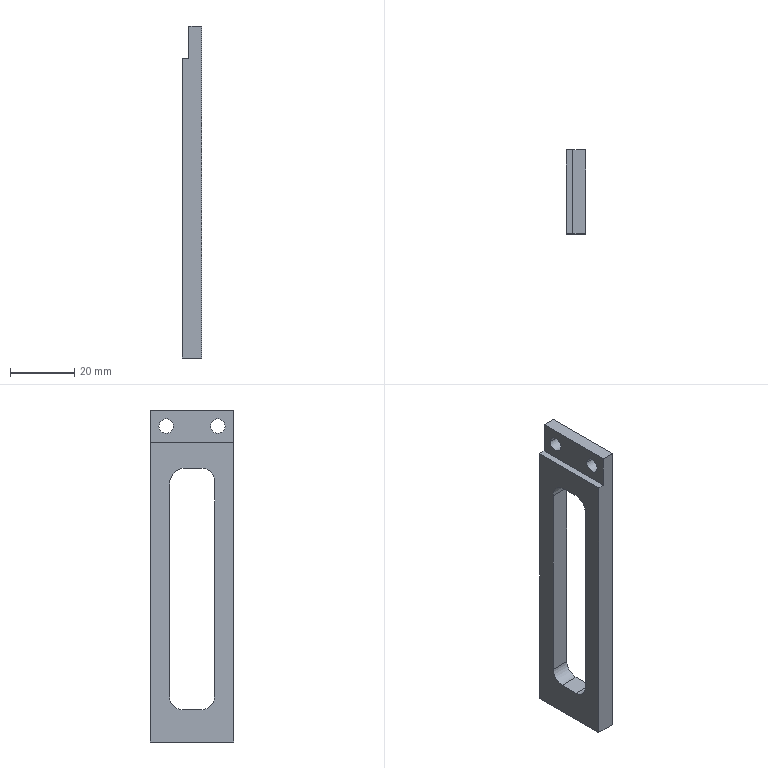Part | NX | 1 solid | 32 faces | box 6 x 26 x 103 mm | volume 9123 mm3 | plane 12 | cylinder 12 | cone 8 | commonest cylinder face diameters 2.5 x4 4.5 x4 8 x3 10 x1
STEP:
#1=CARTESIAN_POINT('',(594.,123.4,-250.82));
#2=VERTEX_POINT('',#1);
#3=CARTESIAN_POINT('',(592.,123.4,-250.82));
#4=VERTEX_POINT('',#3);
#5=CARTESIAN_POINT('',(594.,123.4,-250.82));
#6=DIRECTION('',(-1.,0.,0.));
#7=VECTOR('',#6,1000.);
#8=LINE('',#5,#7);
#9=EDGE_CURVE('',#2,#4,#8,.T.);
#10=ORIENTED_EDGE('',*,*,#9,.T.);
#11=CARTESIAN_POINT('',(592.,123.4,-343.82));
#12=VERTEX_POINT('',#11);
#13=CARTESIAN_POINT('',(592.,123.4,-246.201));
#14=DIRECTION('',(0.,0.,1.));
#15=VECTOR('',#14,1000.);
#16=LINE('',#13,#15);
#17=EDGE_CURVE('',#12,#4,#16,.T.);
#18=ORIENTED_EDGE('',*,*,#17,.F.);
#19=CARTESIAN_POINT('',(598.,123.4,-343.82));
#20=VERTEX_POINT('',#19);
#21=CARTESIAN_POINT('',(594.,123.4,-343.82));
#22=DIRECTION('',(1.,0.,0.));
#23=VECTOR('',#22,1000.);
#24=LINE('',#21,#23);
#25=EDGE_CURVE('',#12,#20,#24,.T.);
#26=ORIENTED_EDGE('',*,*,#25,.T.);
#27=CARTESIAN_POINT('',(598.,123.4,-240.82));
#28=VERTEX_POINT('',#27);
#29=CARTESIAN_POINT('',(598.,123.4,-246.201));
#30=DIRECTION('',(0.,0.,-1.));
#31=VECTOR('',#30,1000.);
#32=LINE('',#29,#31);
#33=EDGE_CURVE('',#28,#20,#32,.T.);
#34=ORIENTED_EDGE('',*,*,#33,.F.);
#35=CARTESIAN_POINT('',(594.,123.4,-240.82));
#36=VERTEX_POINT('',#35);
#37=CARTESIAN_POINT('',(594.,123.4,-240.82));
#38=DIRECTION('',(-1.,0.,0.));
#39=VECTOR('',#38,1000.);
#40=LINE('',#37,#39);
#41=EDGE_CURVE('',#28,#36,#40,.T.);
#42=ORIENTED_EDGE('',*,*,#41,.T.);
#43=CARTESIAN_POINT('',(594.,123.4,-246.201));
#44=DIRECTION('',(0.,0.,1.));
#45=VECTOR('',#44,1000.);
#46=LINE('',#43,#45);
#47=EDGE_CURVE('',#2,#36,#46,.T.);
#48=ORIENTED_EDGE('',*,*,#47,.F.);
#49=EDGE_LOOP('',(#10,#18,#26,#34,#42,#48));
#50=FACE_BOUND('',#49,.T.);
#51=CARTESIAN_POINT('',(594.,123.4,-250.82));
#52=DIRECTION('',(0.,-1.,0.));
#53=DIRECTION('',(0.,0.,-1.));
#54=AXIS2_PLACEMENT_3D('',#51,#52,#53);
#55=PLANE('',#54);
#56=ADVANCED_FACE('',(#50),#55,.T.);
#57=CARTESIAN_POINT('',(592.,149.4,-343.82));
#58=VERTEX_POINT('',#57);
#59=CARTESIAN_POINT('',(598.,149.4,-343.82));
#60=VERTEX_POINT('',#59);
#61=CARTESIAN_POINT('',(594.,149.4,-343.82));
#62=DIRECTION('',(1.,0.,0.));
#63=VECTOR('',#62,1000.);
#64=LINE('',#61,#63);
#65=EDGE_CURVE('',#58,#60,#64,.T.);
#66=ORIENTED_EDGE('',*,*,#65,.T.);
#67=CARTESIAN_POINT('',(598.,141.756,-343.82));
#68=DIRECTION('',(0.,1.,0.));
#69=VECTOR('',#68,1000.);
#70=LINE('',#67,#69);
#71=EDGE_CURVE('',#20,#60,#70,.T.);
#72=ORIENTED_EDGE('',*,*,#71,.F.);
#73=ORIENTED_EDGE('',*,*,#25,.F.);
#74=CARTESIAN_POINT('',(592.,141.756,-343.82));
#75=DIRECTION('',(0.,-1.,0.));
#76=VECTOR('',#75,1000.);
#77=LINE('',#74,#76);
#78=EDGE_CURVE('',#58,#12,#77,.T.);
#79=ORIENTED_EDGE('',*,*,#78,.F.);
#80=EDGE_LOOP('',(#66,#72,#73,#79));
#81=FACE_BOUND('',#80,.T.);
#82=CARTESIAN_POINT('',(596.6,126.9,-343.82));
#83=VERTEX_POINT('',#82);
#84=CARTESIAN_POINT('',(593.2,126.9,-343.82));
#85=VERTEX_POINT('',#84);
#86=CARTESIAN_POINT('',(594.9,126.9,-343.82));
#87=DIRECTION('',(0.,0.,-1.));
#88=DIRECTION('',(0.,-1.,0.));
#89=AXIS2_PLACEMENT_3D('',#86,#87,#88);
#90=CIRCLE('',#89,1.7);
#91=EDGE_CURVE('',#83,#85,#90,.T.);
#92=ORIENTED_EDGE('',*,*,#91,.F.);
#93=CARTESIAN_POINT('',(594.9,126.9,-343.82));
#94=DIRECTION('',(0.,0.,-1.));
#95=DIRECTION('',(0.,-1.,0.));
#96=AXIS2_PLACEMENT_3D('',#93,#94,#95);
#97=CIRCLE('',#96,1.7);
#98=EDGE_CURVE('',#85,#83,#97,.T.);
#99=ORIENTED_EDGE('',*,*,#98,.F.);
#100=EDGE_LOOP('',(#92,#99));
#101=FACE_BOUND('',#100,.T.);
#102=CARTESIAN_POINT('',(596.6,145.9,-343.82));
#103=VERTEX_POINT('',#102);
#104=CARTESIAN_POINT('',(593.2,145.9,-343.82));
#105=VERTEX_POINT('',#104);
#106=CARTESIAN_POINT('',(594.9,145.9,-343.82));
#107=DIRECTION('',(0.,0.,-1.));
#108=DIRECTION('',(0.,-1.,0.));
#109=AXIS2_PLACEMENT_3D('',#106,#107,#108);
#110=CIRCLE('',#109,1.7);
#111=EDGE_CURVE('',#103,#105,#110,.T.);
#112=ORIENTED_EDGE('',*,*,#111,.F.);
#113=CARTESIAN_POINT('',(594.9,145.9,-343.82));
#114=DIRECTION('',(0.,0.,-1.));
#115=DIRECTION('',(0.,-1.,0.));
#116=AXIS2_PLACEMENT_3D('',#113,#114,#115);
#117=CIRCLE('',#116,1.7);
#118=EDGE_CURVE('',#105,#103,#117,.T.);
#119=ORIENTED_EDGE('',*,*,#118,.F.);
#120=EDGE_LOOP('',(#112,#119));
#121=FACE_BOUND('',#120,.T.);
#122=CARTESIAN_POINT('',(594.,146.4,-343.82));
#123=DIRECTION('',(0.,0.,-1.));
#124=DIRECTION('',(0.,-1.,0.));
#125=AXIS2_PLACEMENT_3D('',#122,#123,#124);
#126=PLANE('',#125);
#127=ADVANCED_FACE('',(#81,#101,#121),#126,.T.);
#128=CARTESIAN_POINT('',(594.,149.4,-240.82));
#129=VERTEX_POINT('',#128);
#130=CARTESIAN_POINT('',(594.,149.4,-250.82));
#131=VERTEX_POINT('',#130);
#132=CARTESIAN_POINT('',(594.,149.4,-246.201));
#133=DIRECTION('',(0.,0.,-1.));
#134=VECTOR('',#133,1000.);
#135=LINE('',#132,#134);
#136=EDGE_CURVE('',#129,#131,#135,.T.);
#137=ORIENTED_EDGE('',*,*,#136,.F.);
#138=CARTESIAN_POINT('',(598.,149.4,-240.82));
#139=VERTEX_POINT('',#138);
#140=CARTESIAN_POINT('',(594.,149.4,-240.82));
#141=DIRECTION('',(1.,0.,0.));
#142=VECTOR('',#141,1000.);
#143=LINE('',#140,#142);
#144=EDGE_CURVE('',#129,#139,#143,.T.);
#145=ORIENTED_EDGE('',*,*,#144,.T.);
#146=CARTESIAN_POINT('',(598.,149.4,-246.201));
#147=DIRECTION('',(0.,0.,1.));
#148=VECTOR('',#147,1000.);
#149=LINE('',#146,#148);
#150=EDGE_CURVE('',#60,#139,#149,.T.);
#151=ORIENTED_EDGE('',*,*,#150,.F.);
#152=ORIENTED_EDGE('',*,*,#65,.F.);
#153=CARTESIAN_POINT('',(592.,149.4,-250.82));
#154=VERTEX_POINT('',#153);
#155=CARTESIAN_POINT('',(592.,149.4,-246.201));
#156=DIRECTION('',(0.,0.,-1.));
#157=VECTOR('',#156,1000.);
#158=LINE('',#155,#157);
#159=EDGE_CURVE('',#154,#58,#158,.T.);
#160=ORIENTED_EDGE('',*,*,#159,.F.);
#161=CARTESIAN_POINT('',(594.,149.4,-250.82));
#162=DIRECTION('',(1.,0.,0.));
#163=VECTOR('',#162,1000.);
#164=LINE('',#161,#163);
#165=EDGE_CURVE('',#154,#131,#164,.T.);
#166=ORIENTED_EDGE('',*,*,#165,.T.);
#167=EDGE_LOOP('',(#137,#145,#151,#152,#160,#166));
#168=FACE_BOUND('',#167,.T.);
#169=CARTESIAN_POINT('',(594.,149.4,-240.82));
#170=DIRECTION('',(0.,1.,0.));
#171=DIRECTION('',(1.,0.,0.));
#172=AXIS2_PLACEMENT_3D('',#169,#170,#171);
#173=PLANE('',#172);
#174=ADVANCED_FACE('',(#168),#173,.T.);
#175=CARTESIAN_POINT('',(594.,141.756,-240.82));
#176=DIRECTION('',(0.,1.,0.));
#177=VECTOR('',#176,1000.);
#178=LINE('',#175,#177);
#179=EDGE_CURVE('',#36,#129,#178,.T.);
#180=ORIENTED_EDGE('',*,*,#179,.F.);
#181=ORIENTED_EDGE('',*,*,#41,.F.);
#182=CARTESIAN_POINT('',(598.,141.756,-240.82));
#183=DIRECTION('',(0.,-1.,0.));
#184=VECTOR('',#183,1000.);
#185=LINE('',#182,#184);
#186=EDGE_CURVE('',#139,#28,#185,.T.);
#187=ORIENTED_EDGE('',*,*,#186,.F.);
#188=ORIENTED_EDGE('',*,*,#144,.F.);
#189=EDGE_LOOP('',(#180,#181,#187,#188));
#190=FACE_BOUND('',#189,.T.);
#191=CARTESIAN_POINT('',(594.,126.4,-240.82));
#192=DIRECTION('',(0.,0.,1.));
#193=DIRECTION('',(1.,0.,0.));
#194=AXIS2_PLACEMENT_3D('',#191,#192,#193);
#195=PLANE('',#194);
#196=ADVANCED_FACE('',(#190),#195,.T.);
#197=CARTESIAN_POINT('',(592.,141.756,-250.82));
#198=DIRECTION('',(0.,1.,0.));
#199=VECTOR('',#198,1000.);
#200=LINE('',#197,#199);
#201=EDGE_CURVE('',#4,#154,#200,.T.);
#202=ORIENTED_EDGE('',*,*,#201,.T.);
#203=ORIENTED_EDGE('',*,*,#159,.T.);
#204=ORIENTED_EDGE('',*,*,#78,.T.);
#205=ORIENTED_EDGE('',*,*,#17,.T.);
#206=EDGE_LOOP('',(#202,#203,#204,#205));
#207=FACE_BOUND('',#206,.T.);
#208=CARTESIAN_POINT('',(592.,129.4,-329.82));
#209=VERTEX_POINT('',#208);
#210=CARTESIAN_POINT('',(592.,129.4,-262.82));
#211=VERTEX_POINT('',#210);
#212=CARTESIAN_POINT('',(592.,129.4,-246.201));
#213=DIRECTION('',(0.,0.,1.));
#214=VECTOR('',#213,1000.);
#215=LINE('',#212,#214);
#216=EDGE_CURVE('',#209,#211,#215,.T.);
#217=ORIENTED_EDGE('',*,*,#216,.F.);
#218=CARTESIAN_POINT('',(592.,133.4,-333.82));
#219=VERTEX_POINT('',#218);
#220=CARTESIAN_POINT('',(592.,133.4,-329.82));
#221=DIRECTION('',(-1.,0.,0.));
#222=DIRECTION('',(0.,-1.,0.));
#223=AXIS2_PLACEMENT_3D('',#220,#221,#222);
#224=CIRCLE('',#223,4.);
#225=EDGE_CURVE('',#219,#209,#224,.T.);
#226=ORIENTED_EDGE('',*,*,#225,.F.);
#227=CARTESIAN_POINT('',(592.,139.4,-333.82));
#228=VERTEX_POINT('',#227);
#229=CARTESIAN_POINT('',(592.,141.756,-333.82));
#230=DIRECTION('',(0.,-1.,0.));
#231=VECTOR('',#230,1000.);
#232=LINE('',#229,#231);
#233=EDGE_CURVE('',#228,#219,#232,.T.);
#234=ORIENTED_EDGE('',*,*,#233,.F.);
#235=CARTESIAN_POINT('',(592.,143.4,-329.82));
#236=VERTEX_POINT('',#235);
#237=CARTESIAN_POINT('',(592.,139.4,-329.82));
#238=DIRECTION('',(1.,0.,0.));
#239=DIRECTION('',(0.,1.,0.));
#240=AXIS2_PLACEMENT_3D('',#237,#238,#239);
#241=CIRCLE('',#240,4.);
#242=EDGE_CURVE('',#228,#236,#241,.T.);
#243=ORIENTED_EDGE('',*,*,#242,.T.);
#244=CARTESIAN_POINT('',(592.,143.4,-263.82));
#245=VERTEX_POINT('',#244);
#246=CARTESIAN_POINT('',(592.,143.4,-246.201));
#247=DIRECTION('',(0.,0.,-1.));
#248=VECTOR('',#247,1000.);
#249=LINE('',#246,#248);
#250=EDGE_CURVE('',#245,#236,#249,.T.);
#251=ORIENTED_EDGE('',*,*,#250,.F.);
#252=CARTESIAN_POINT('',(592.,138.4,-258.82));
#253=VERTEX_POINT('',#252);
#254=CARTESIAN_POINT('',(592.,138.4,-263.82));
#255=DIRECTION('',(1.,0.,0.));
#256=DIRECTION('',(0.,1.,0.));
#257=AXIS2_PLACEMENT_3D('',#254,#255,#256);
#258=CIRCLE('',#257,5.);
#259=EDGE_CURVE('',#245,#253,#258,.T.);
#260=ORIENTED_EDGE('',*,*,#259,.T.);
#261=CARTESIAN_POINT('',(592.,133.4,-258.82));
#262=VERTEX_POINT('',#261);
#263=CARTESIAN_POINT('',(592.,141.756,-258.82));
#264=DIRECTION('',(0.,1.,0.));
#265=VECTOR('',#264,1000.);
#266=LINE('',#263,#265);
#267=EDGE_CURVE('',#262,#253,#266,.T.);
#268=ORIENTED_EDGE('',*,*,#267,.F.);
#269=CARTESIAN_POINT('',(592.,133.4,-262.82));
#270=DIRECTION('',(1.,0.,0.));
#271=DIRECTION('',(0.,1.,0.));
#272=AXIS2_PLACEMENT_3D('',#269,#270,#271);
#273=CIRCLE('',#272,4.);
#274=EDGE_CURVE('',#262,#211,#273,.T.);
#275=ORIENTED_EDGE('',*,*,#274,.T.);
#276=EDGE_LOOP('',(#217,#226,#234,#243,#251,#260,#268,#275));
#277=FACE_BOUND('',#276,.T.);
#278=CARTESIAN_POINT('',(592.,137.557,-267.86));
#279=DIRECTION('',(-1.,0.,0.));
#280=DIRECTION('',(0.,0.,1.));
#281=AXIS2_PLACEMENT_3D('',#278,#279,#280);
#282=PLANE('',#281);
#283=ADVANCED_FACE('',(#207,#277),#282,.T.);
#284=CARTESIAN_POINT('',(598.,133.4,-258.82));
#285=VERTEX_POINT('',#284);
#286=CARTESIAN_POINT('',(594.,133.4,-258.82));
#287=DIRECTION('',(1.,0.,0.));
#288=VECTOR('',#287,1000.);
#289=LINE('',#286,#288);
#290=EDGE_CURVE('',#262,#285,#289,.T.);
#291=ORIENTED_EDGE('',*,*,#290,.F.);
#292=ORIENTED_EDGE('',*,*,#267,.T.);
#293=CARTESIAN_POINT('',(598.,138.4,-258.82));
#294=VERTEX_POINT('',#293);
#295=CARTESIAN_POINT('',(594.,138.4,-258.82));
#296=DIRECTION('',(1.,0.,0.));
#297=VECTOR('',#296,1000.);
#298=LINE('',#295,#297);
#299=EDGE_CURVE('',#253,#294,#298,.T.);
#300=ORIENTED_EDGE('',*,*,#299,.T.);
#301=CARTESIAN_POINT('',(598.,141.756,-258.82));
#302=DIRECTION('',(0.,-1.,0.));
#303=VECTOR('',#302,1000.);
#304=LINE('',#301,#303);
#305=EDGE_CURVE('',#294,#285,#304,.T.);
#306=ORIENTED_EDGE('',*,*,#305,.T.);
#307=EDGE_LOOP('',(#291,#292,#300,#306));
#308=FACE_BOUND('',#307,.T.);
#309=CARTESIAN_POINT('',(591.4,129.4,-258.82));
#310=DIRECTION('',(0.,0.,1.));
#311=DIRECTION('',(1.,0.,0.));
#312=AXIS2_PLACEMENT_3D('',#309,#310,#311);
#313=PLANE('',#312);
#314=ADVANCED_FACE('',(#308),#313,.F.);
#315=CARTESIAN_POINT('',(598.,129.4,-329.82));
#316=VERTEX_POINT('',#315);
#317=CARTESIAN_POINT('',(594.,129.4,-329.82));
#318=DIRECTION('',(-1.,0.,0.));
#319=VECTOR('',#318,1000.);
#320=LINE('',#317,#319);
#321=EDGE_CURVE('',#316,#209,#320,.T.);
#322=ORIENTED_EDGE('',*,*,#321,.T.);
#323=ORIENTED_EDGE('',*,*,#216,.T.);
#324=CARTESIAN_POINT('',(598.,129.4,-262.82));
#325=VERTEX_POINT('',#324);
#326=CARTESIAN_POINT('',(594.,129.4,-262.82));
#327=DIRECTION('',(1.,0.,0.));
#328=VECTOR('',#327,1000.);
#329=LINE('',#326,#328);
#330=EDGE_CURVE('',#211,#325,#329,.T.);
#331=ORIENTED_EDGE('',*,*,#330,.T.);
#332=CARTESIAN_POINT('',(598.,129.4,-246.201));
#333=DIRECTION('',(0.,0.,-1.));
#334=VECTOR('',#333,1000.);
#335=LINE('',#332,#334);
#336=EDGE_CURVE('',#325,#316,#335,.T.);
#337=ORIENTED_EDGE('',*,*,#336,.T.);
#338=EDGE_LOOP('',(#322,#323,#331,#337));
#339=FACE_BOUND('',#338,.T.);
#340=CARTESIAN_POINT('',(591.4,129.4,-331.82));
#341=DIRECTION('',(0.,-1.,0.));
#342=DIRECTION('',(0.,0.,-1.));
#343=AXIS2_PLACEMENT_3D('',#340,#341,#342);
#344=PLANE('',#343);
#345=ADVANCED_FACE('',(#339),#344,.F.);
#346=CARTESIAN_POINT('',(598.,143.4,-329.82));
#347=VERTEX_POINT('',#346);
#348=CARTESIAN_POINT('',(594.,143.4,-329.82));
#349=DIRECTION('',(1.,0.,0.));
#350=VECTOR('',#349,1000.);
#351=LINE('',#348,#350);
#352=EDGE_CURVE('',#236,#347,#351,.T.);
#353=ORIENTED_EDGE('',*,*,#352,.T.);
#354=CARTESIAN_POINT('',(598.,143.4,-263.82));
#355=VERTEX_POINT('',#354);
#356=CARTESIAN_POINT('',(598.,143.4,-246.201));
#357=DIRECTION('',(0.,0.,1.));
#358=VECTOR('',#357,1000.);
#359=LINE('',#356,#358);
#360=EDGE_CURVE('',#347,#355,#359,.T.);
#361=ORIENTED_EDGE('',*,*,#360,.T.);
#362=CARTESIAN_POINT('',(594.,143.4,-263.82));
#363=DIRECTION('',(1.,0.,0.));
#364=VECTOR('',#363,1000.);
#365=LINE('',#362,#364);
#366=EDGE_CURVE('',#245,#355,#365,.T.);
#367=ORIENTED_EDGE('',*,*,#366,.F.);
#368=ORIENTED_EDGE('',*,*,#250,.T.);
#369=EDGE_LOOP('',(#353,#361,#367,#368));
#370=FACE_BOUND('',#369,.T.);
#371=CARTESIAN_POINT('',(591.4,143.4,-258.82));
#372=DIRECTION('',(0.,1.,0.));
#373=DIRECTION('',(1.,0.,0.));
#374=AXIS2_PLACEMENT_3D('',#371,#372,#373);
#375=PLANE('',#374);
#376=ADVANCED_FACE('',(#370),#375,.F.);
#377=CARTESIAN_POINT('',(598.,133.4,-333.82));
#378=VERTEX_POINT('',#377);
#379=CARTESIAN_POINT('',(598.,139.4,-333.82));
#380=VERTEX_POINT('',#379);
#381=CARTESIAN_POINT('',(598.,141.756,-333.82));
#382=DIRECTION('',(0.,1.,0.));
#383=VECTOR('',#382,1000.);
#384=LINE('',#381,#383);
#385=EDGE_CURVE('',#378,#380,#384,.T.);
#386=ORIENTED_EDGE('',*,*,#385,.T.);
#387=CARTESIAN_POINT('',(594.,139.4,-333.82));
#388=DIRECTION('',(1.,0.,0.));
#389=VECTOR('',#388,1000.);
#390=LINE('',#387,#389);
#391=EDGE_CURVE('',#228,#380,#390,.T.);
#392=ORIENTED_EDGE('',*,*,#391,.F.);
#393=ORIENTED_EDGE('',*,*,#233,.T.);
#394=CARTESIAN_POINT('',(594.,133.4,-333.82));
#395=DIRECTION('',(-1.,0.,0.));
#396=VECTOR('',#395,1000.);
#397=LINE('',#394,#396);
#398=EDGE_CURVE('',#378,#219,#397,.T.);
#399=ORIENTED_EDGE('',*,*,#398,.F.);
#400=EDGE_LOOP('',(#386,#392,#393,#399));
#401=FACE_BOUND('',#400,.T.);
#402=CARTESIAN_POINT('',(591.4,143.4,-333.82));
#403=DIRECTION('',(0.,0.,-1.));
#404=DIRECTION('',(0.,-1.,0.));
#405=AXIS2_PLACEMENT_3D('',#402,#403,#404);
#406=PLANE('',#405);
#407=ADVANCED_FACE('',(#401),#406,.F.);
#408=ORIENTED_EDGE('',*,*,#366,.T.);
#409=CARTESIAN_POINT('',(598.,138.4,-263.82));
#410=DIRECTION('',(1.,0.,0.));
#411=DIRECTION('',(0.,1.,0.));
#412=AXIS2_PLACEMENT_3D('',#409,#410,#411);
#413=CIRCLE('',#412,5.);
#414=EDGE_CURVE('',#355,#294,#413,.T.);
#415=ORIENTED_EDGE('',*,*,#414,.T.);
#416=ORIENTED_EDGE('',*,*,#299,.F.);
#417=ORIENTED_EDGE('',*,*,#259,.F.);
#418=EDGE_LOOP('',(#408,#415,#416,#417));
#419=FACE_BOUND('',#418,.T.);
#420=CARTESIAN_POINT('',(594.,138.4,-263.82));
#421=DIRECTION('',(1.,0.,0.));
#422=DIRECTION('',(0.,1.,0.));
#423=AXIS2_PLACEMENT_3D('',#420,#421,#422);
#424=CYLINDRICAL_SURFACE('',#423,5.);
#425=ADVANCED_FACE('',(#419),#424,.F.);
#426=ORIENTED_EDGE('',*,*,#290,.T.);
#427=CARTESIAN_POINT('',(598.,133.4,-262.82));
#428=DIRECTION('',(1.,0.,0.));
#429=DIRECTION('',(0.,1.,0.));
#430=AXIS2_PLACEMENT_3D('',#427,#428,#429);
#431=CIRCLE('',#430,4.);
#432=EDGE_CURVE('',#285,#325,#431,.T.);
#433=ORIENTED_EDGE('',*,*,#432,.T.);
#434=ORIENTED_EDGE('',*,*,#330,.F.);
#435=ORIENTED_EDGE('',*,*,#274,.F.);
#436=EDGE_LOOP('',(#426,#433,#434,#435));
#437=FACE_BOUND('',#436,.T.);
#438=CARTESIAN_POINT('',(594.,133.4,-262.82));
#439=DIRECTION('',(1.,0.,0.));
#440=DIRECTION('',(0.,1.,0.));
#441=AXIS2_PLACEMENT_3D('',#438,#439,#440);
#442=CYLINDRICAL_SURFACE('',#441,4.);
#443=ADVANCED_FACE('',(#437),#442,.F.);
#444=ORIENTED_EDGE('',*,*,#352,.F.);
#445=ORIENTED_EDGE('',*,*,#242,.F.);
#446=ORIENTED_EDGE('',*,*,#391,.T.);
#447=CARTESIAN_POINT('',(598.,139.4,-329.82));
#448=DIRECTION('',(1.,0.,0.));
#449=DIRECTION('',(0.,1.,0.));
#450=AXIS2_PLACEMENT_3D('',#447,#448,#449);
#451=CIRCLE('',#450,4.);
#452=EDGE_CURVE('',#380,#347,#451,.T.);
#453=ORIENTED_EDGE('',*,*,#452,.T.);
#454=EDGE_LOOP('',(#444,#445,#446,#453));
#455=FACE_BOUND('',#454,.T.);
#456=CARTESIAN_POINT('',(594.,139.4,-329.82));
#457=DIRECTION('',(1.,0.,0.));
#458=DIRECTION('',(0.,1.,0.));
#459=AXIS2_PLACEMENT_3D('',#456,#457,#458);
#460=CYLINDRICAL_SURFACE('',#459,4.);
#461=ADVANCED_FACE('',(#455),#460,.F.);
#462=ORIENTED_EDGE('',*,*,#321,.F.);
#463=CARTESIAN_POINT('',(598.,133.4,-329.82));
#464=DIRECTION('',(-1.,0.,0.));
#465=DIRECTION('',(0.,-1.,0.));
#466=AXIS2_PLACEMENT_3D('',#463,#464,#465);
#467=CIRCLE('',#466,4.);
#468=EDGE_CURVE('',#378,#316,#467,.T.);
#469=ORIENTED_EDGE('',*,*,#468,.F.);
#470=ORIENTED_EDGE('',*,*,#398,.T.);
#471=ORIENTED_EDGE('',*,*,#225,.T.);
#472=EDGE_LOOP('',(#462,#469,#470,#471));
#473=FACE_BOUND('',#472,.T.);
#474=CARTESIAN_POINT('',(594.,133.4,-329.82));
#475=DIRECTION('',(-1.,0.,0.));
#476=DIRECTION('',(0.,-1.,0.));
#477=AXIS2_PLACEMENT_3D('',#474,#475,#476);
#478=CYLINDRICAL_SURFACE('',#477,4.);
#479=ADVANCED_FACE('',(#473),#478,.F.);
#480=CARTESIAN_POINT('',(596.15,126.9,-343.56));
#481=VERTEX_POINT('',#480);
#482=CARTESIAN_POINT('',(594.9,125.65,-343.56));
#483=VERTEX_POINT('',#482);
#484=CARTESIAN_POINT('',(594.9,126.9,-343.56));
#485=DIRECTION('',(0.,0.,-1.));
#486=DIRECTION('',(0.,-1.,0.));
#487=AXIS2_PLACEMENT_3D('',#484,#485,#486);
#488=CIRCLE('',#487,1.25);
#489=EDGE_CURVE('',#481,#483,#488,.T.);
#490=ORIENTED_EDGE('',*,*,#489,.T.);
#491=CARTESIAN_POINT('',(594.9,125.65,-334.82));
#492=VERTEX_POINT('',#491);
#493=CARTESIAN_POINT('',(594.9,125.65,-343.82));
#494=DIRECTION('',(0.,0.,-1.));
#495=VECTOR('',#494,1000.);
#496=LINE('',#493,#495);
#497=EDGE_CURVE('',#483,#492,#496,.F.);
#498=ORIENTED_EDGE('',*,*,#497,.T.);
#499=CARTESIAN_POINT('',(596.15,126.9,-334.82));
#500=VERTEX_POINT('',#499);
#501=CARTESIAN_POINT('',(594.9,126.9,-334.82));
#502=DIRECTION('',(0.,0.,-1.));
#503=DIRECTION('',(0.,-1.,0.));
#504=AXIS2_PLACEMENT_3D('',#501,#502,#503);
#505=CIRCLE('',#504,1.25);
#506=EDGE_CURVE('',#500,#492,#505,.T.);
#507=ORIENTED_EDGE('',*,*,#506,.F.);
#508=CARTESIAN_POINT('',(594.9,128.15,-334.82));
#509=VERTEX_POINT('',#508);
#510=CARTESIAN_POINT('',(594.9,126.9,-334.82));
#511=DIRECTION('',(0.,0.,-1.));
#512=DIRECTION('',(0.,-1.,0.));
#513=AXIS2_PLACEMENT_3D('',#510,#511,#512);
#514=CIRCLE('',#513,1.25);
#515=EDGE_CURVE('',#509,#500,#514,.T.);
#516=ORIENTED_EDGE('',*,*,#515,.F.);
#517=CARTESIAN_POINT('',(594.9,128.15,-343.56));
#518=VERTEX_POINT('',#517);
#519=CARTESIAN_POINT('',(594.9,128.15,-343.82));
#520=DIRECTION('',(0.,0.,-1.));
#521=VECTOR('',#520,1000.);
#522=LINE('',#519,#521);
#523=EDGE_CURVE('',#518,#509,#522,.F.);
#524=ORIENTED_EDGE('',*,*,#523,.F.);
#525=CARTESIAN_POINT('',(594.9,126.9,-343.56));
#526=DIRECTION('',(0.,0.,-1.));
#527=DIRECTION('',(0.,-1.,0.));
#528=AXIS2_PLACEMENT_3D('',#525,#526,#527);
#529=CIRCLE('',#528,1.25);
#530=EDGE_CURVE('',#518,#481,#529,.T.);
#531=ORIENTED_EDGE('',*,*,#530,.T.);
#532=EDGE_LOOP('',(#490,#498,#507,#516,#524,#531));
#533=FACE_BOUND('',#532,.T.);
#534=CARTESIAN_POINT('',(594.9,126.9,-343.82));
#535=DIRECTION('',(0.,0.,-1.));
#536=DIRECTION('',(0.,-1.,0.));
#537=AXIS2_PLACEMENT_3D('',#534,#535,#536);
#538=CYLINDRICAL_SURFACE('',#537,1.25);
#539=ADVANCED_FACE('',(#533),#538,.F.);
#540=ORIENTED_EDGE('',*,*,#71,.T.);
#541=ORIENTED_EDGE('',*,*,#150,.T.);
#542=ORIENTED_EDGE('',*,*,#186,.T.);
#543=ORIENTED_EDGE('',*,*,#33,.T.);
#544=EDGE_LOOP('',(#540,#541,#542,#543));
#545=FACE_BOUND('',#544,.T.);
#546=CARTESIAN_POINT('',(598.,142.15,-245.82));
#547=VERTEX_POINT('',#546);
#548=CARTESIAN_POINT('',(598.,146.65,-245.82));
#549=VERTEX_POINT('',#548);
#550=CARTESIAN_POINT('',(598.,144.4,-245.82));
#551=DIRECTION('',(1.,0.,0.));
#552=DIRECTION('',(0.,1.,0.));
#553=AXIS2_PLACEMENT_3D('',#550,#551,#552);
#554=CIRCLE('',#553,2.25);
#555=EDGE_CURVE('',#547,#549,#554,.T.);
#556=ORIENTED_EDGE('',*,*,#555,.F.);
#557=CARTESIAN_POINT('',(598.,144.4,-245.82));
#558=DIRECTION('',(1.,0.,0.));
#559=DIRECTION('',(0.,1.,0.));
#560=AXIS2_PLACEMENT_3D('',#557,#558,#559);
#561=CIRCLE('',#560,2.25);
#562=EDGE_CURVE('',#549,#547,#561,.T.);
#563=ORIENTED_EDGE('',*,*,#562,.F.);
#564=EDGE_LOOP('',(#556,#563));
#565=FACE_BOUND('',#564,.T.);
#566=ORIENTED_EDGE('',*,*,#336,.F.);
#567=ORIENTED_EDGE('',*,*,#432,.F.);
#568=ORIENTED_EDGE('',*,*,#305,.F.);
#569=ORIENTED_EDGE('',*,*,#414,.F.);
#570=ORIENTED_EDGE('',*,*,#360,.F.);
#571=ORIENTED_EDGE('',*,*,#452,.F.);
#572=ORIENTED_EDGE('',*,*,#385,.F.);
#573=ORIENTED_EDGE('',*,*,#468,.T.);
#574=EDGE_LOOP('',(#566,#567,#568,#569,#570,#571,#572,#573));
#575=FACE_BOUND('',#574,.T.);
#576=CARTESIAN_POINT('',(598.,130.65,-245.82));
#577=VERTEX_POINT('',#576);
#578=CARTESIAN_POINT('',(598.,126.15,-245.82));
#579=VERTEX_POINT('',#578);
#580=CARTESIAN_POINT('',(598.,128.4,-245.82));
#581=DIRECTION('',(1.,0.,0.));
#582=DIRECTION('',(0.,1.,0.));
#583=AXIS2_PLACEMENT_3D('',#580,#581,#582);
#584=CIRCLE('',#583,2.25);
#585=EDGE_CURVE('',#577,#579,#584,.T.);
#586=ORIENTED_EDGE('',*,*,#585,.F.);
#587=CARTESIAN_POINT('',(598.,128.4,-245.82));
#588=DIRECTION('',(1.,0.,0.));
#589=DIRECTION('',(0.,1.,0.));
#590=AXIS2_PLACEMENT_3D('',#587,#588,#589);
#591=CIRCLE('',#590,2.25);
#592=EDGE_CURVE('',#579,#577,#591,.T.);
#593=ORIENTED_EDGE('',*,*,#592,.F.);
#594=EDGE_LOOP('',(#586,#593));
#595=FACE_BOUND('',#594,.T.);
#596=CARTESIAN_POINT('',(598.,141.756,-246.201));
#597=DIRECTION('',(1.,0.,0.));
#598=DIRECTION('',(0.,1.,0.));
#599=AXIS2_PLACEMENT_3D('',#596,#597,#598);
#600=PLANE('',#599);
#601=ADVANCED_FACE('',(#545,#565,#575,#595),#600,.T.);
#602=CARTESIAN_POINT('',(593.65,126.9,-334.82));
#603=VERTEX_POINT('',#602);
#604=CARTESIAN_POINT('',(594.9,126.9,-334.82));
#605=DIRECTION('',(0.,0.,-1.));
#606=DIRECTION('',(0.,-1.,0.));
#607=AXIS2_PLACEMENT_3D('',#604,#605,#606);
#608=CIRCLE('',#607,1.25);
#609=EDGE_CURVE('',#492,#603,#608,.T.);
#610=ORIENTED_EDGE('',*,*,#609,.T.);
#611=CARTESIAN_POINT('',(594.9,126.9,-334.069));
#612=VERTEX_POINT('',#611);
#613=CARTESIAN_POINT('',(593.65,126.9,-334.82));
#614=DIRECTION('',(-0.8572,0.,-0.515));
#615=VECTOR('',#614,1000.);
#616=LINE('',#613,#615);
#617=EDGE_CURVE('',#612,#603,#616,.T.);
#618=ORIENTED_EDGE('',*,*,#617,.F.);
#619=CARTESIAN_POINT('',(596.15,126.9,-334.82));
#620=DIRECTION('',(0.8572,0.,-0.515));
#621=VECTOR('',#620,1000.);
#622=LINE('',#619,#621);
#623=EDGE_CURVE('',#612,#500,#622,.T.);
#624=ORIENTED_EDGE('',*,*,#623,.T.);
#625=ORIENTED_EDGE('',*,*,#506,.T.);
#626=EDGE_LOOP('',(#610,#618,#624,#625));
#627=FACE_BOUND('',#626,.T.);
#628=CARTESIAN_POINT('',(594.9,126.9,-334.82));
#629=DIRECTION('',(0.,0.,-1.));
#630=DIRECTION('',(-1.,0.,0.));
#631=AXIS2_PLACEMENT_3D('',#628,#629,#630);
#632=CONICAL_SURFACE('',#631,1.25,1.03);
#633=ADVANCED_FACE('',(#627),#632,.F.);
#634=ORIENTED_EDGE('',*,*,#489,.F.);
#635=CARTESIAN_POINT('',(596.15,126.9,-343.56));
#636=DIRECTION('',(0.866,0.,-0.5));
#637=VECTOR('',#636,1000.);
#638=LINE('',#635,#637);
#639=EDGE_CURVE('',#481,#83,#638,.T.);
#640=ORIENTED_EDGE('',*,*,#639,.T.);
#641=ORIENTED_EDGE('',*,*,#91,.T.);
#642=CARTESIAN_POINT('',(593.65,126.9,-343.56));
#643=VERTEX_POINT('',#642);
#644=CARTESIAN_POINT('',(593.65,126.9,-343.56));
#645=DIRECTION('',(-0.866,0.,-0.5));
#646=VECTOR('',#645,1000.);
#647=LINE('',#644,#646);
#648=EDGE_CURVE('',#643,#85,#647,.T.);
#649=ORIENTED_EDGE('',*,*,#648,.F.);
#650=CARTESIAN_POINT('',(594.9,126.9,-343.56));
#651=DIRECTION('',(0.,0.,-1.));
#652=DIRECTION('',(0.,-1.,0.));
#653=AXIS2_PLACEMENT_3D('',#650,#651,#652);
#654=CIRCLE('',#653,1.25);
#655=EDGE_CURVE('',#483,#643,#654,.T.);
#656=ORIENTED_EDGE('',*,*,#655,.F.);
#657=EDGE_LOOP('',(#634,#640,#641,#649,#656));
#658=FACE_BOUND('',#657,.T.);
#659=CARTESIAN_POINT('',(594.9,126.9,-343.56));
#660=DIRECTION('',(0.,0.,-1.));
#661=DIRECTION('',(-1.,0.,0.));
#662=AXIS2_PLACEMENT_3D('',#659,#660,#661);
#663=CONICAL_SURFACE('',#662,1.25,1.047);
#664=ADVANCED_FACE('',(#658),#663,.F.);
#665=CARTESIAN_POINT('',(593.65,145.9,-334.82));
#666=VERTEX_POINT('',#665);
#667=CARTESIAN_POINT('',(594.9,147.15,-334.82));
#668=VERTEX_POINT('',#667);
#669=CARTESIAN_POINT('',(594.9,145.9,-334.82));
#670=DIRECTION('',(0.,0.,-1.));
#671=DIRECTION('',(0.,-1.,0.));
#672=AXIS2_PLACEMENT_3D('',#669,#670,#671);
#673=CIRCLE('',#672,1.25);
#674=EDGE_CURVE('',#666,#668,#673,.T.);
#675=ORIENTED_EDGE('',*,*,#674,.F.);
#676=CARTESIAN_POINT('',(594.9,144.65,-334.82));
#677=VERTEX_POINT('',#676);
#678=CARTESIAN_POINT('',(594.9,145.9,-334.82));
#679=DIRECTION('',(0.,0.,-1.));
#680=DIRECTION('',(0.,-1.,0.));
#681=AXIS2_PLACEMENT_3D('',#678,#679,#680);
#682=CIRCLE('',#681,1.25);
#683=EDGE_CURVE('',#677,#666,#682,.T.);
#684=ORIENTED_EDGE('',*,*,#683,.F.);
#685=CARTESIAN_POINT('',(594.9,144.65,-343.56));
#686=VERTEX_POINT('',#685);
#687=CARTESIAN_POINT('',(594.9,144.65,-343.82));
#688=DIRECTION('',(0.,0.,-1.));
#689=VECTOR('',#688,1000.);
#690=LINE('',#687,#689);
#691=EDGE_CURVE('',#686,#677,#690,.F.);
#692=ORIENTED_EDGE('',*,*,#691,.F.);
#693=CARTESIAN_POINT('',(593.65,145.9,-343.56));
#694=VERTEX_POINT('',#693);
#695=CARTESIAN_POINT('',(594.9,145.9,-343.56));
#696=DIRECTION('',(0.,0.,-1.));
#697=DIRECTION('',(0.,-1.,0.));
#698=AXIS2_PLACEMENT_3D('',#695,#696,#697);
#699=CIRCLE('',#698,1.25);
#700=EDGE_CURVE('',#686,#694,#699,.T.);
#701=ORIENTED_EDGE('',*,*,#700,.T.);
#702=CARTESIAN_POINT('',(594.9,147.15,-343.56));
#703=VERTEX_POINT('',#702);
#704=CARTESIAN_POINT('',(594.9,145.9,-343.56));
#705=DIRECTION('',(0.,0.,-1.));
#706=DIRECTION('',(0.,-1.,0.));
#707=AXIS2_PLACEMENT_3D('',#704,#705,#706);
#708=CIRCLE('',#707,1.25);
#709=EDGE_CURVE('',#694,#703,#708,.T.);
#710=ORIENTED_EDGE('',*,*,#709,.T.);
#711=CARTESIAN_POINT('',(594.9,147.15,-343.82));
#712=DIRECTION('',(0.,0.,-1.));
#713=VECTOR('',#712,1000.);
#714=LINE('',#711,#713);
#715=EDGE_CURVE('',#703,#668,#714,.F.);
#716=ORIENTED_EDGE('',*,*,#715,.T.);
#717=EDGE_LOOP('',(#675,#684,#692,#701,#710,#716));
#718=FACE_BOUND('',#717,.T.);
#719=CARTESIAN_POINT('',(594.9,145.9,-343.82));
#720=DIRECTION('',(0.,0.,-1.));
#721=DIRECTION('',(0.,-1.,0.));
#722=AXIS2_PLACEMENT_3D('',#719,#720,#721);
#723=CYLINDRICAL_SURFACE('',#722,1.25);
#724=ADVANCED_FACE('',(#718),#723,.F.);
#725=CARTESIAN_POINT('',(594.,146.65,-245.82));
#726=VERTEX_POINT('',#725);
#727=CARTESIAN_POINT('',(594.,142.15,-245.82));
#728=VERTEX_POINT('',#727);
#729=CARTESIAN_POINT('',(594.,144.4,-245.82));
#730=DIRECTION('',(1.,0.,0.));
#731=DIRECTION('',(0.,1.,0.));
#732=AXIS2_PLACEMENT_3D('',#729,#730,#731);
#733=CIRCLE('',#732,2.25);
#734=EDGE_CURVE('',#726,#728,#733,.T.);
#735=ORIENTED_EDGE('',*,*,#734,.F.);
#736=CARTESIAN_POINT('',(594.,146.65,-245.82));
#737=DIRECTION('',(1.,0.,0.));
#738=VECTOR('',#737,1000.);
#739=LINE('',#736,#738);
#740=EDGE_CURVE('',#726,#549,#739,.T.);
#741=ORIENTED_EDGE('',*,*,#740,.T.);
#742=ORIENTED_EDGE('',*,*,#562,.T.);
#743=CARTESIAN_POINT('',(594.,142.15,-245.82));
#744=DIRECTION('',(1.,0.,0.));
#745=VECTOR('',#744,1000.);
#746=LINE('',#743,#745);
#747=EDGE_CURVE('',#728,#547,#746,.T.);
#748=ORIENTED_EDGE('',*,*,#747,.F.);
#749=EDGE_LOOP('',(#735,#741,#742,#748));
#750=FACE_BOUND('',#749,.T.);
#751=CARTESIAN_POINT('',(594.,144.4,-245.82));
#752=DIRECTION('',(1.,0.,0.));
#753=DIRECTION('',(0.,1.,0.));
#754=AXIS2_PLACEMENT_3D('',#751,#752,#753);
#755=CYLINDRICAL_SURFACE('',#754,2.25);
#756=ADVANCED_FACE('',(#750),#755,.F.);
#757=CARTESIAN_POINT('',(594.9,145.9,-334.069));
#758=VERTEX_POINT('',#757);
#759=CARTESIAN_POINT('',(596.15,145.9,-334.82));
#760=VERTEX_POINT('',#759);
#761=CARTESIAN_POINT('',(596.15,145.9,-334.82));
#762=DIRECTION('',(0.8572,0.,-0.515));
#763=VECTOR('',#762,1000.);
#764=LINE('',#761,#763);
#765=EDGE_CURVE('',#758,#760,#764,.T.);
#766=ORIENTED_EDGE('',*,*,#765,.T.);
#767=CARTESIAN_POINT('',(594.9,145.9,-334.82));
#768=DIRECTION('',(0.,0.,-1.));
#769=DIRECTION('',(0.,-1.,0.));
#770=AXIS2_PLACEMENT_3D('',#767,#768,#769);
#771=CIRCLE('',#770,1.25);
#772=EDGE_CURVE('',#760,#677,#771,.T.);
#773=ORIENTED_EDGE('',*,*,#772,.T.);
#774=ORIENTED_EDGE('',*,*,#683,.T.);
#775=CARTESIAN_POINT('',(593.65,145.9,-334.82));
#776=DIRECTION('',(-0.8572,0.,-0.515));
#777=VECTOR('',#776,1000.);
#778=LINE('',#775,#777);
#779=EDGE_CURVE('',#758,#666,#778,.T.);
#780=ORIENTED_EDGE('',*,*,#779,.F.);
#781=EDGE_LOOP('',(#766,#773,#774,#780));
#782=FACE_BOUND('',#781,.T.);
#783=CARTESIAN_POINT('',(594.9,145.9,-334.82));
#784=DIRECTION('',(0.,0.,-1.));
#785=DIRECTION('',(-1.,0.,0.));
#786=AXIS2_PLACEMENT_3D('',#783,#784,#785);
#787=CONICAL_SURFACE('',#786,1.25,1.03);
#788=ADVANCED_FACE('',(#782),#787,.F.);
#789=CARTESIAN_POINT('',(596.15,145.9,-343.56));
#790=VERTEX_POINT('',#789);
#791=CARTESIAN_POINT('',(594.9,145.9,-343.56));
#792=DIRECTION('',(0.,0.,-1.));
#793=DIRECTION('',(0.,-1.,0.));
#794=AXIS2_PLACEMENT_3D('',#791,#792,#793);
#795=CIRCLE('',#794,1.25);
#796=EDGE_CURVE('',#703,#790,#795,.T.);
#797=ORIENTED_EDGE('',*,*,#796,.F.);
#798=ORIENTED_EDGE('',*,*,#709,.F.);
#799=CARTESIAN_POINT('',(593.65,145.9,-343.56));
#800=DIRECTION('',(-0.866,0.,-0.5));
#801=VECTOR('',#800,1000.);
#802=LINE('',#799,#801);
#803=EDGE_CURVE('',#105,#694,#802,.F.);
#804=ORIENTED_EDGE('',*,*,#803,.F.);
#805=ORIENTED_EDGE('',*,*,#118,.T.);
#806=CARTESIAN_POINT('',(596.15,145.9,-343.56));
#807=DIRECTION('',(0.866,0.,-0.5));
#808=VECTOR('',#807,1000.);
#809=LINE('',#806,#808);
#810=EDGE_CURVE('',#103,#790,#809,.F.);
#811=ORIENTED_EDGE('',*,*,#810,.T.);
#812=EDGE_LOOP('',(#797,#798,#804,#805,#811));
#813=FACE_BOUND('',#812,.T.);
#814=CARTESIAN_POINT('',(594.9,145.9,-343.56));
#815=DIRECTION('',(0.,0.,-1.));
#816=DIRECTION('',(-1.,0.,0.));
#817=AXIS2_PLACEMENT_3D('',#814,#815,#816);
#818=CONICAL_SURFACE('',#817,1.25,1.047);
#819=ADVANCED_FACE('',(#813),#818,.F.);
#820=CARTESIAN_POINT('',(594.,141.756,-250.82));
#821=DIRECTION('',(0.,1.,0.));
#822=VECTOR('',#821,1000.);
#823=LINE('',#820,#822);
#824=EDGE_CURVE('',#2,#131,#823,.T.);
#825=ORIENTED_EDGE('',*,*,#824,.T.);
#826=ORIENTED_EDGE('',*,*,#165,.F.);
#827=ORIENTED_EDGE('',*,*,#201,.F.);
#828=ORIENTED_EDGE('',*,*,#9,.F.);
#829=EDGE_LOOP('',(#825,#826,#827,#828));
#830=FACE_BOUND('',#829,.T.);
#831=CARTESIAN_POINT('',(594.,146.4,-250.82));
#832=DIRECTION('',(0.,0.,1.));
#833=DIRECTION('',(1.,0.,0.));
#834=AXIS2_PLACEMENT_3D('',#831,#832,#833);
#835=PLANE('',#834);
#836=ADVANCED_FACE('',(#830),#835,.T.);
#837=ORIENTED_EDGE('',*,*,#585,.T.);
#838=CARTESIAN_POINT('',(594.,126.15,-245.82));
#839=VERTEX_POINT('',#838);
#840=CARTESIAN_POINT('',(594.,126.15,-245.82));
#841=DIRECTION('',(1.,0.,0.));
#842=VECTOR('',#841,1000.);
#843=LINE('',#840,#842);
#844=EDGE_CURVE('',#579,#839,#843,.F.);
#845=ORIENTED_EDGE('',*,*,#844,.T.);
#846=CARTESIAN_POINT('',(594.,130.65,-245.82));
#847=VERTEX_POINT('',#846);
#848=CARTESIAN_POINT('',(594.,128.4,-245.82));
#849=DIRECTION('',(1.,0.,0.));
#850=DIRECTION('',(0.,1.,0.));
#851=AXIS2_PLACEMENT_3D('',#848,#849,#850);
#852=CIRCLE('',#851,2.25);
#853=EDGE_CURVE('',#847,#839,#852,.T.);
#854=ORIENTED_EDGE('',*,*,#853,.F.);
#855=CARTESIAN_POINT('',(594.,130.65,-245.82));
#856=DIRECTION('',(1.,0.,0.));
#857=VECTOR('',#856,1000.);
#858=LINE('',#855,#857);
#859=EDGE_CURVE('',#577,#847,#858,.F.);
#860=ORIENTED_EDGE('',*,*,#859,.F.);
#861=EDGE_LOOP('',(#837,#845,#854,#860));
#862=FACE_BOUND('',#861,.T.);
#863=CARTESIAN_POINT('',(594.,128.4,-245.82));
#864=DIRECTION('',(1.,0.,0.));
#865=DIRECTION('',(0.,1.,0.));
#866=AXIS2_PLACEMENT_3D('',#863,#864,#865);
#867=CYLINDRICAL_SURFACE('',#866,2.25);
#868=ADVANCED_FACE('',(#862),#867,.F.);
#869=ORIENTED_EDGE('',*,*,#824,.F.);
#870=ORIENTED_EDGE('',*,*,#47,.T.);
#871=ORIENTED_EDGE('',*,*,#179,.T.);
#872=ORIENTED_EDGE('',*,*,#136,.T.);
#873=EDGE_LOOP('',(#869,#870,#871,#872));
#874=FACE_BOUND('',#873,.T.);
#875=ORIENTED_EDGE('',*,*,#734,.T.);
#876=CARTESIAN_POINT('',(594.,144.4,-245.82));
#877=DIRECTION('',(1.,0.,0.));
#878=DIRECTION('',(0.,1.,0.));
#879=AXIS2_PLACEMENT_3D('',#876,#877,#878);
#880=CIRCLE('',#879,2.25);
#881=EDGE_CURVE('',#728,#726,#880,.T.);
#882=ORIENTED_EDGE('',*,*,#881,.T.);
#883=EDGE_LOOP('',(#875,#882));
#884=FACE_BOUND('',#883,.T.);
#885=CARTESIAN_POINT('',(594.,128.4,-245.82));
#886=DIRECTION('',(1.,0.,0.));
#887=DIRECTION('',(0.,1.,0.));
#888=AXIS2_PLACEMENT_3D('',#885,#886,#887);
#889=CIRCLE('',#888,2.25);
#890=EDGE_CURVE('',#839,#847,#889,.T.);
#891=ORIENTED_EDGE('',*,*,#890,.T.);
#892=ORIENTED_EDGE('',*,*,#853,.T.);
#893=EDGE_LOOP('',(#891,#892));
#894=FACE_BOUND('',#893,.T.);
#895=CARTESIAN_POINT('',(594.,141.756,-246.201));
#896=DIRECTION('',(1.,0.,0.));
#897=DIRECTION('',(0.,1.,0.));
#898=AXIS2_PLACEMENT_3D('',#895,#896,#897);
#899=PLANE('',#898);
#900=ADVANCED_FACE('',(#874,#884,#894),#899,.F.);
#901=ORIENTED_EDGE('',*,*,#639,.F.);
#902=ORIENTED_EDGE('',*,*,#530,.F.);
#903=CARTESIAN_POINT('',(594.9,126.9,-343.56));
#904=DIRECTION('',(0.,0.,-1.));
#905=DIRECTION('',(0.,-1.,0.));
#906=AXIS2_PLACEMENT_3D('',#903,#904,#905);
#907=CIRCLE('',#906,1.25);
#908=EDGE_CURVE('',#643,#518,#907,.T.);
#909=ORIENTED_EDGE('',*,*,#908,.F.);
#910=ORIENTED_EDGE('',*,*,#648,.T.);
#911=ORIENTED_EDGE('',*,*,#98,.T.);
#912=EDGE_LOOP('',(#901,#902,#909,#910,#911));
#913=FACE_BOUND('',#912,.T.);
#914=CARTESIAN_POINT('',(594.9,126.9,-343.56));
#915=DIRECTION('',(0.,0.,-1.));
#916=DIRECTION('',(-1.,0.,0.));
#917=AXIS2_PLACEMENT_3D('',#914,#915,#916);
#918=CONICAL_SURFACE('',#917,1.25,1.047);
#919=ADVANCED_FACE('',(#913),#918,.F.);
#920=ORIENTED_EDGE('',*,*,#555,.T.);
#921=ORIENTED_EDGE('',*,*,#740,.F.);
#922=ORIENTED_EDGE('',*,*,#881,.F.);
#923=ORIENTED_EDGE('',*,*,#747,.T.);
#924=EDGE_LOOP('',(#920,#921,#922,#923));
#925=FACE_BOUND('',#924,.T.);
#926=CARTESIAN_POINT('',(594.,144.4,-245.82));
#927=DIRECTION('',(1.,0.,0.));
#928=DIRECTION('',(0.,1.,0.));
#929=AXIS2_PLACEMENT_3D('',#926,#927,#928);
#930=CYLINDRICAL_SURFACE('',#929,2.25);
#931=ADVANCED_FACE('',(#925),#930,.F.);
#932=ORIENTED_EDGE('',*,*,#674,.T.);
#933=CARTESIAN_POINT('',(594.9,145.9,-334.82));
#934=DIRECTION('',(0.,0.,-1.));
#935=DIRECTION('',(0.,-1.,0.));
#936=AXIS2_PLACEMENT_3D('',#933,#934,#935);
#937=CIRCLE('',#936,1.25);
#938=EDGE_CURVE('',#668,#760,#937,.T.);
#939=ORIENTED_EDGE('',*,*,#938,.T.);
#940=ORIENTED_EDGE('',*,*,#765,.F.);
#941=ORIENTED_EDGE('',*,*,#779,.T.);
#942=EDGE_LOOP('',(#932,#939,#940,#941));
#943=FACE_BOUND('',#942,.T.);
#944=CARTESIAN_POINT('',(594.9,145.9,-334.82));
#945=DIRECTION('',(0.,0.,-1.));
#946=DIRECTION('',(-1.,0.,0.));
#947=AXIS2_PLACEMENT_3D('',#944,#945,#946);
#948=CONICAL_SURFACE('',#947,1.25,1.03);
#949=ADVANCED_FACE('',(#943),#948,.F.);
#950=ORIENTED_EDGE('',*,*,#796,.T.);
#951=CARTESIAN_POINT('',(594.9,145.9,-343.56));
#952=DIRECTION('',(0.,0.,-1.));
#953=DIRECTION('',(0.,-1.,0.));
#954=AXIS2_PLACEMENT_3D('',#951,#952,#953);
#955=CIRCLE('',#954,1.25);
#956=EDGE_CURVE('',#790,#686,#955,.T.);
#957=ORIENTED_EDGE('',*,*,#956,.T.);
#958=ORIENTED_EDGE('',*,*,#691,.T.);
#959=ORIENTED_EDGE('',*,*,#772,.F.);
#960=ORIENTED_EDGE('',*,*,#938,.F.);
#961=ORIENTED_EDGE('',*,*,#715,.F.);
#962=EDGE_LOOP('',(#950,#957,#958,#959,#960,#961));
#963=FACE_BOUND('',#962,.T.);
#964=CARTESIAN_POINT('',(594.9,145.9,-343.82));
#965=DIRECTION('',(0.,0.,-1.));
#966=DIRECTION('',(0.,-1.,0.));
#967=AXIS2_PLACEMENT_3D('',#964,#965,#966);
#968=CYLINDRICAL_SURFACE('',#967,1.25);
#969=ADVANCED_FACE('',(#963),#968,.F.);
#970=ORIENTED_EDGE('',*,*,#111,.T.);
#971=ORIENTED_EDGE('',*,*,#803,.T.);
#972=ORIENTED_EDGE('',*,*,#700,.F.);
#973=ORIENTED_EDGE('',*,*,#956,.F.);
#974=ORIENTED_EDGE('',*,*,#810,.F.);
#975=EDGE_LOOP('',(#970,#971,#972,#973,#974));
#976=FACE_BOUND('',#975,.T.);
#977=CARTESIAN_POINT('',(594.9,145.9,-343.56));
#978=DIRECTION('',(0.,0.,-1.));
#979=DIRECTION('',(-1.,0.,0.));
#980=AXIS2_PLACEMENT_3D('',#977,#978,#979);
#981=CONICAL_SURFACE('',#980,1.25,1.047);
#982=ADVANCED_FACE('',(#976),#981,.F.);
#983=ORIENTED_EDGE('',*,*,#623,.F.);
#984=ORIENTED_EDGE('',*,*,#617,.T.);
#985=CARTESIAN_POINT('',(594.9,126.9,-334.82));
#986=DIRECTION('',(0.,0.,-1.));
#987=DIRECTION('',(0.,-1.,0.));
#988=AXIS2_PLACEMENT_3D('',#985,#986,#987);
#989=CIRCLE('',#988,1.25);
#990=EDGE_CURVE('',#603,#509,#989,.T.);
#991=ORIENTED_EDGE('',*,*,#990,.T.);
#992=ORIENTED_EDGE('',*,*,#515,.T.);
#993=EDGE_LOOP('',(#983,#984,#991,#992));
#994=FACE_BOUND('',#993,.T.);
#995=CARTESIAN_POINT('',(594.9,126.9,-334.82));
#996=DIRECTION('',(0.,0.,-1.));
#997=DIRECTION('',(-1.,0.,0.));
#998=AXIS2_PLACEMENT_3D('',#995,#996,#997);
#999=CONICAL_SURFACE('',#998,1.25,1.03);
#1000=ADVANCED_FACE('',(#994),#999,.F.);
#1001=ORIENTED_EDGE('',*,*,#890,.F.);
#1002=ORIENTED_EDGE('',*,*,#844,.F.);
#1003=ORIENTED_EDGE('',*,*,#592,.T.);
#1004=ORIENTED_EDGE('',*,*,#859,.T.);
#1005=EDGE_LOOP('',(#1001,#1002,#1003,#1004));
#1006=FACE_BOUND('',#1005,.T.);
#1007=CARTESIAN_POINT('',(594.,128.4,-245.82));
#1008=DIRECTION('',(1.,0.,0.));
#1009=DIRECTION('',(0.,1.,0.));
#1010=AXIS2_PLACEMENT_3D('',#1007,#1008,#1009);
#1011=CYLINDRICAL_SURFACE('',#1010,2.25);
#1012=ADVANCED_FACE('',(#1006),#1011,.F.);
#1013=ORIENTED_EDGE('',*,*,#609,.F.);
#1014=ORIENTED_EDGE('',*,*,#497,.F.);
#1015=ORIENTED_EDGE('',*,*,#655,.T.);
#1016=ORIENTED_EDGE('',*,*,#908,.T.);
#1017=ORIENTED_EDGE('',*,*,#523,.T.);
#1018=ORIENTED_EDGE('',*,*,#990,.F.);
#1019=EDGE_LOOP('',(#1013,#1014,#1015,#1016,#1017,#1018));
#1020=FACE_BOUND('',#1019,.T.);
#1021=CARTESIAN_POINT('',(594.9,126.9,-343.82));
#1022=DIRECTION('',(0.,0.,-1.));
#1023=DIRECTION('',(0.,-1.,0.));
#1024=AXIS2_PLACEMENT_3D('',#1021,#1022,#1023);
#1025=CYLINDRICAL_SURFACE('',#1024,1.25);
#1026=ADVANCED_FACE('',(#1020),#1025,.F.);
#1027=CLOSED_SHELL('',(#56,#127,#174,#196,#283,#314,#345,#376,#407,#425,#443,#461,#479,#539,#601,#633,#664,#724,#756,#788,#819,#836,#868,#900,#919,#931,#949,#969,#982,#1000,#1012,#1026));
#1028=MANIFOLD_SOLID_BREP('',#1027);
#1029=(LENGTH_UNIT()NAMED_UNIT(*)SI_UNIT(.MILLI.,.METRE.));
#1030=UNCERTAINTY_MEASURE_WITH_UNIT(LENGTH_MEASURE(0.00001),#1029,'','');
#1031=(NAMED_UNIT(*)PLANE_ANGLE_UNIT()SI_UNIT($,.RADIAN.));
#1032=(NAMED_UNIT(*)SI_UNIT($,.STERADIAN.)SOLID_ANGLE_UNIT());
#1033=(GEOMETRIC_REPRESENTATION_CONTEXT(3)GLOBAL_UNCERTAINTY_ASSIGNED_CONTEXT((#1030))GLOBAL_UNIT_ASSIGNED_CONTEXT((#1029,#1031,#1032))REPRESENTATION_CONTEXT('',''));
#1034=ADVANCED_BREP_SHAPE_REPRESENTATION('',(#1028),#1033);